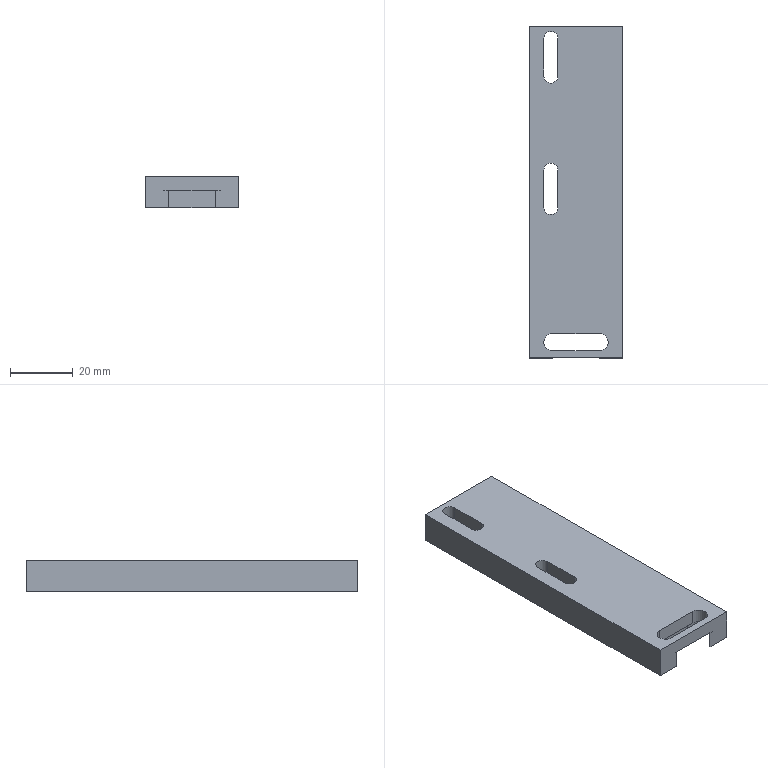CAM job | NX | 3-axis milling | part box 30 x 106 x 10 mm | stock box 35 x 111 x 12 mm
Tools:
number,name,description,diameter,corner_radius,flute_length,length,flutes
4,D4,平底铣刀-粗,4.0,0.0,25.0,75.0,2
6,D6,平底铣刀-粗,6.0,0.0,25.0,75.0,2
9,D10,平底铣刀-粗,10.0,0.0,35.0,75.0,2
11,D4-J,平底铣刀-精,4.0,0.0,50.0,75.0,2
7,D6-J,平底铣刀-精,6.0,0.0,25.0,75.0,2
10,D10-J,平底铣刀-精,10.0,0.0,35.0,75.0,2
1,D80R0.8飞刀,圆鼻刀-粗,80.0,0.8,50.0,75.0,2
1,D80R0.8飞刀-J,圆鼻刀-精,80.0,0.8,50.0,75.0,2
2,D6倒角刀,倒角刀,6.0,0.0,3.0,25.0,2
Operations:
program,operation,operation_type,tool,method,geometry_group,spindle_rpm,surface_speed,feed_per_tooth,feed_cut,feed_plunge,cut_length_mm,path_length_mm,cut_time_min,machine_time_min
B,底壁铣飞面一刀开粗_COPY,VolumeBased25DMillingOperation,D80R0.8飞刀,分层开粗-切深K-步距G,W-B,2800.0,703.696,0.5357,3000.0,100.0,856.776,1581.735,0.2856,0.3581
B,底壁铣飞面一刀精光_COPY,VolumeBased25DMillingOperation,D80R0.8飞刀-J,侧刃精光-切深K-步距G,W-B,4000.0,1005.28,0.125,1000.0,100.0,213.998,309.998,0.214,0.2236
B,C0.3平面去毛刺6X45L__COPY,SurfaceContour,D6倒角刀,爬面_倒角-切深0-步距G,W-B,8000.0,150.796,0.0938,1500.0,90.0,399.649,694.75,0.267,0.2965
A,顶面,FaceMilling,D80R0.8飞刀,侧刃精光-切深K-步距G,W-A,4000.0,1005.31,0.125,1000.0,100.0,200.0,236.0,0.2,0.2036
A,外形粗_2,VolumeBased25DMillingOperation,D10,METHOD,W-A,8000.0,251.327,0.3125,5000.0,80.0,4562.177,4610.677,0.9124,0.9173
A,底壁粗_1,VolumeBased25DMillingOperation,D6,METHOD,W-A,6000.0,113.0,0.2083,3500.0,100.0,1055.386,1185.715,0.3015,0.3146
A,通腰槽粗_1,VolumeBased25DMillingOperation,D4,METHOD,W-A,6000.0,75.398,0.1,1200.0,100.0,2148.158,2286.658,1.79,1.804
A,通腰槽粗_2,VolumeBased25DMillingOperation,D4,METHOD,W-A,6000.0,75.398,0.1,1200.0,100.0,717.284,771.284,0.5977,0.6031
A,底精_1,VolumeBased25DMillingOperation,D6-J,METHOD,W-A,6000.0,113.0,0.2083,1200.0,100.0,77.746,127.746,0.0648,0.0698
A,底侧精_3,VolumeBased25DMillingOperation,D6-J,METHOD,W-A,6000.0,113.0,0.2083,1200.0,100.0,47.847,97.837,0.0399,0.0449
A,腰槽精_1,VolumeBased25DMillingOperation,D4-J,METHOD,W-A,6000.0,113.0,0.0417,500.0,100.0,111.197,294.497,0.2224,0.2407
A,腰槽精_2,VolumeBased25DMillingOperation,D4-J,METHOD,W-A,6000.0,113.0,0.0417,500.0,100.0,36.941,95.941,0.0739,0.0798
A,仅选体,SurfaceContour,D6倒角刀,METHOD,W-A,8000.0,150.796,0.1875,3000.0,100.0,481.546,763.857,0.1605,0.1887
A,外形半精_2,VolumeBased25DMillingOperation,D10-J,METHOD,W-A,8000.0,251.327,0.0625,1000.0,100.0,308.374,367.374,0.3084,0.3143